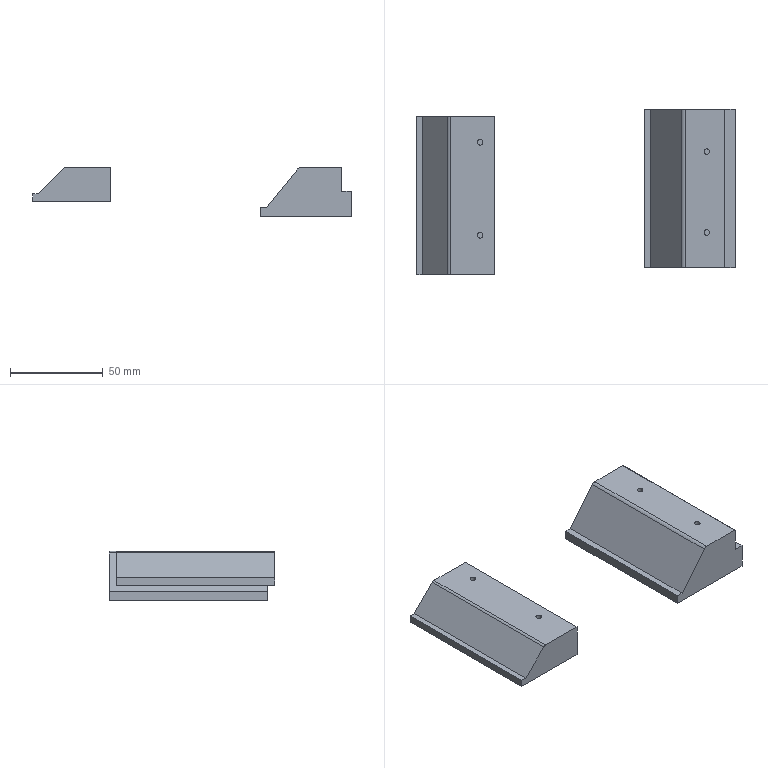Part | NX | 2 solids | 29 faces | box 171.319 x 88.841 x 26.598 mm | volume 135499 mm3 | plane 22 | cylinder 7 | commonest cylinder face diameters 3 x4 1 x1 4 x1 5 x1
STEP:
#1=CARTESIAN_POINT('',(92.218,-38.659,-21.598));
#2=VERTEX_POINT('',#1);
#3=CARTESIAN_POINT('',(92.218,-38.659,-26.598));
#4=VERTEX_POINT('',#3);
#5=CARTESIAN_POINT('',(92.218,-38.659,-21.598));
#6=DIRECTION('',(0.,0.,-1.));
#7=VECTOR('',#6,1000.);
#8=LINE('',#5,#7);
#9=EDGE_CURVE('',#2,#4,#8,.T.);
#10=ORIENTED_EDGE('',*,*,#9,.F.);
#11=CARTESIAN_POINT('',(92.218,46.341,-21.598));
#12=VERTEX_POINT('',#11);
#13=CARTESIAN_POINT('',(92.218,46.341,-21.598));
#14=DIRECTION('',(0.,-1.,0.));
#15=VECTOR('',#14,1000.);
#16=LINE('',#13,#15);
#17=EDGE_CURVE('',#12,#2,#16,.T.);
#18=ORIENTED_EDGE('',*,*,#17,.F.);
#19=CARTESIAN_POINT('',(92.218,46.341,-26.598));
#20=VERTEX_POINT('',#19);
#21=CARTESIAN_POINT('',(92.218,46.341,-21.598));
#22=DIRECTION('',(0.,0.,-1.));
#23=VECTOR('',#22,1000.);
#24=LINE('',#21,#23);
#25=EDGE_CURVE('',#12,#20,#24,.T.);
#26=ORIENTED_EDGE('',*,*,#25,.T.);
#27=CARTESIAN_POINT('',(92.218,46.341,-26.598));
#28=DIRECTION('',(0.,-1.,0.));
#29=VECTOR('',#28,1000.);
#30=LINE('',#27,#29);
#31=EDGE_CURVE('',#20,#4,#30,.T.);
#32=ORIENTED_EDGE('',*,*,#31,.T.);
#33=EDGE_LOOP('',(#10,#18,#26,#32));
#34=FACE_BOUND('',#33,.T.);
#35=CARTESIAN_POINT('',(92.218,46.341,-21.598));
#36=DIRECTION('',(-1.,0.,0.));
#37=DIRECTION('',(0.,-1.,0.));
#38=AXIS2_PLACEMENT_3D('',#35,#36,#37);
#39=PLANE('',#38);
#40=ADVANCED_FACE('',(#34),#39,.T.);
#41=CARTESIAN_POINT('',(141.218,-38.659,-26.598));
#42=VERTEX_POINT('',#41);
#43=CARTESIAN_POINT('',(92.218,-38.659,-26.598));
#44=DIRECTION('',(1.,0.,0.));
#45=VECTOR('',#44,1000.);
#46=LINE('',#43,#45);
#47=EDGE_CURVE('',#4,#42,#46,.T.);
#48=ORIENTED_EDGE('',*,*,#47,.F.);
#49=ORIENTED_EDGE('',*,*,#31,.F.);
#50=CARTESIAN_POINT('',(141.218,46.341,-26.598));
#51=VERTEX_POINT('',#50);
#52=CARTESIAN_POINT('',(92.218,46.341,-26.598));
#53=DIRECTION('',(1.,0.,0.));
#54=VECTOR('',#53,1000.);
#55=LINE('',#52,#54);
#56=EDGE_CURVE('',#20,#51,#55,.T.);
#57=ORIENTED_EDGE('',*,*,#56,.T.);
#58=CARTESIAN_POINT('',(141.218,46.341,-26.598));
#59=DIRECTION('',(0.,-1.,0.));
#60=VECTOR('',#59,1000.);
#61=LINE('',#58,#60);
#62=EDGE_CURVE('',#51,#42,#61,.T.);
#63=ORIENTED_EDGE('',*,*,#62,.T.);
#64=EDGE_LOOP('',(#48,#49,#57,#63));
#65=FACE_BOUND('',#64,.T.);
#66=CARTESIAN_POINT('',(92.218,46.341,-26.598));
#67=DIRECTION('',(0.,0.,-1.));
#68=DIRECTION('',(0.,1.,0.));
#69=AXIS2_PLACEMENT_3D('',#66,#67,#68);
#70=PLANE('',#69);
#71=ADVANCED_FACE('',(#65),#70,.T.);
#72=CARTESIAN_POINT('',(141.218,-38.659,-13.));
#73=VERTEX_POINT('',#72);
#74=CARTESIAN_POINT('',(141.218,-38.659,-26.598));
#75=DIRECTION('',(0.,0.,1.));
#76=VECTOR('',#75,1000.);
#77=LINE('',#74,#76);
#78=EDGE_CURVE('',#42,#73,#77,.T.);
#79=ORIENTED_EDGE('',*,*,#78,.F.);
#80=ORIENTED_EDGE('',*,*,#62,.F.);
#81=CARTESIAN_POINT('',(141.218,46.341,-13.));
#82=VERTEX_POINT('',#81);
#83=CARTESIAN_POINT('',(141.218,46.341,-26.598));
#84=DIRECTION('',(0.,0.,1.));
#85=VECTOR('',#84,1000.);
#86=LINE('',#83,#85);
#87=EDGE_CURVE('',#51,#82,#86,.T.);
#88=ORIENTED_EDGE('',*,*,#87,.T.);
#89=CARTESIAN_POINT('',(141.218,46.341,-13.));
#90=DIRECTION('',(0.,-1.,0.));
#91=VECTOR('',#90,1000.);
#92=LINE('',#89,#91);
#93=EDGE_CURVE('',#82,#73,#92,.T.);
#94=ORIENTED_EDGE('',*,*,#93,.T.);
#95=EDGE_LOOP('',(#79,#80,#88,#94));
#96=FACE_BOUND('',#95,.T.);
#97=CARTESIAN_POINT('',(141.218,46.341,-26.598));
#98=DIRECTION('',(1.,0.,0.));
#99=DIRECTION('',(0.,1.,0.));
#100=AXIS2_PLACEMENT_3D('',#97,#98,#99);
#101=PLANE('',#100);
#102=ADVANCED_FACE('',(#96),#101,.T.);
#103=CARTESIAN_POINT('',(136.064,-38.659,-13.));
#104=VERTEX_POINT('',#103);
#105=CARTESIAN_POINT('',(141.218,-38.659,-13.));
#106=DIRECTION('',(-1.,0.,0.));
#107=VECTOR('',#106,1000.);
#108=LINE('',#105,#107);
#109=EDGE_CURVE('',#73,#104,#108,.T.);
#110=ORIENTED_EDGE('',*,*,#109,.F.);
#111=ORIENTED_EDGE('',*,*,#93,.F.);
#112=CARTESIAN_POINT('',(136.064,46.341,-13.));
#113=VERTEX_POINT('',#112);
#114=CARTESIAN_POINT('',(141.218,46.341,-13.));
#115=DIRECTION('',(-1.,0.,0.));
#116=VECTOR('',#115,1000.);
#117=LINE('',#114,#116);
#118=EDGE_CURVE('',#82,#113,#117,.T.);
#119=ORIENTED_EDGE('',*,*,#118,.T.);
#120=CARTESIAN_POINT('',(136.064,46.341,-13.));
#121=DIRECTION('',(0.,-1.,0.));
#122=VECTOR('',#121,1000.);
#123=LINE('',#120,#122);
#124=EDGE_CURVE('',#113,#104,#123,.T.);
#125=ORIENTED_EDGE('',*,*,#124,.T.);
#126=EDGE_LOOP('',(#110,#111,#119,#125));
#127=FACE_BOUND('',#126,.T.);
#128=CARTESIAN_POINT('',(141.218,46.341,-13.));
#129=DIRECTION('',(0.,0.,1.));
#130=DIRECTION('',(0.,-1.,0.));
#131=AXIS2_PLACEMENT_3D('',#128,#129,#130);
#132=PLANE('',#131);
#133=ADVANCED_FACE('',(#127),#132,.T.);
#134=CARTESIAN_POINT('',(136.064,-38.659,-0.5));
#135=VERTEX_POINT('',#134);
#136=CARTESIAN_POINT('',(136.064,-38.659,-13.));
#137=DIRECTION('',(0.,0.,1.));
#138=VECTOR('',#137,1000.);
#139=LINE('',#136,#138);
#140=EDGE_CURVE('',#104,#135,#139,.T.);
#141=ORIENTED_EDGE('',*,*,#140,.F.);
#142=ORIENTED_EDGE('',*,*,#124,.F.);
#143=CARTESIAN_POINT('',(136.064,46.341,-0.5));
#144=VERTEX_POINT('',#143);
#145=CARTESIAN_POINT('',(136.064,46.341,-13.));
#146=DIRECTION('',(0.,0.,1.));
#147=VECTOR('',#146,1000.);
#148=LINE('',#145,#147);
#149=EDGE_CURVE('',#113,#144,#148,.T.);
#150=ORIENTED_EDGE('',*,*,#149,.T.);
#151=CARTESIAN_POINT('',(136.064,46.341,-0.5));
#152=DIRECTION('',(0.,-1.,0.));
#153=VECTOR('',#152,1000.);
#154=LINE('',#151,#153);
#155=EDGE_CURVE('',#144,#135,#154,.T.);
#156=ORIENTED_EDGE('',*,*,#155,.T.);
#157=EDGE_LOOP('',(#141,#142,#150,#156));
#158=FACE_BOUND('',#157,.T.);
#159=CARTESIAN_POINT('',(136.064,46.341,-13.));
#160=DIRECTION('',(1.,0.,0.));
#161=DIRECTION('',(0.,1.,0.));
#162=AXIS2_PLACEMENT_3D('',#159,#160,#161);
#163=PLANE('',#162);
#164=ADVANCED_FACE('',(#158),#163,.T.);
#165=CARTESIAN_POINT('',(135.564,-38.659,0.));
#166=VERTEX_POINT('',#165);
#167=CARTESIAN_POINT('',(135.564,-38.659,-0.5));
#168=DIRECTION('',(0.,-1.,0.));
#169=DIRECTION('',(1.,0.,0.));
#170=AXIS2_PLACEMENT_3D('',#167,#168,#169);
#171=CIRCLE('',#170,0.5);
#172=EDGE_CURVE('',#135,#166,#171,.T.);
#173=ORIENTED_EDGE('',*,*,#172,.F.);
#174=ORIENTED_EDGE('',*,*,#155,.F.);
#175=CARTESIAN_POINT('',(135.564,46.341,0.));
#176=VERTEX_POINT('',#175);
#177=CARTESIAN_POINT('',(135.564,46.341,-0.5));
#178=DIRECTION('',(0.,-1.,0.));
#179=DIRECTION('',(1.,0.,0.));
#180=AXIS2_PLACEMENT_3D('',#177,#178,#179);
#181=CIRCLE('',#180,0.5);
#182=EDGE_CURVE('',#144,#176,#181,.T.);
#183=ORIENTED_EDGE('',*,*,#182,.T.);
#184=CARTESIAN_POINT('',(135.564,46.341,0.));
#185=DIRECTION('',(0.,-1.,0.));
#186=VECTOR('',#185,1000.);
#187=LINE('',#184,#186);
#188=EDGE_CURVE('',#176,#166,#187,.T.);
#189=ORIENTED_EDGE('',*,*,#188,.T.);
#190=EDGE_LOOP('',(#173,#174,#183,#189));
#191=FACE_BOUND('',#190,.T.);
#192=CARTESIAN_POINT('',(135.564,46.341,-0.5));
#193=DIRECTION('',(0.,-1.,0.));
#194=DIRECTION('',(1.,0.,0.));
#195=AXIS2_PLACEMENT_3D('',#192,#193,#194);
#196=CYLINDRICAL_SURFACE('',#195,0.5);
#197=ADVANCED_FACE('',(#191),#196,.T.);
#198=CARTESIAN_POINT('',(127.424,23.591,0.));
#199=VERTEX_POINT('',#198);
#200=CARTESIAN_POINT('',(125.924,23.591,0.));
#201=DIRECTION('',(0.,0.,1.));
#202=DIRECTION('',(1.,0.,0.));
#203=AXIS2_PLACEMENT_3D('',#200,#201,#202);
#204=CIRCLE('',#203,1.5);
#205=EDGE_CURVE('',#199,#199,#204,.T.);
#206=ORIENTED_EDGE('',*,*,#205,.F.);
#207=EDGE_LOOP('',(#206));
#208=FACE_BOUND('',#207,.T.);
#209=CARTESIAN_POINT('',(127.424,-19.908,0.));
#210=VERTEX_POINT('',#209);
#211=CARTESIAN_POINT('',(125.924,-19.908,0.));
#212=DIRECTION('',(0.,0.,1.));
#213=DIRECTION('',(1.,0.,0.));
#214=AXIS2_PLACEMENT_3D('',#211,#212,#213);
#215=CIRCLE('',#214,1.5);
#216=EDGE_CURVE('',#210,#210,#215,.T.);
#217=ORIENTED_EDGE('',*,*,#216,.F.);
#218=EDGE_LOOP('',(#217));
#219=FACE_BOUND('',#218,.T.);
#220=CARTESIAN_POINT('',(114.318,-38.659,0.));
#221=VERTEX_POINT('',#220);
#222=CARTESIAN_POINT('',(135.564,-38.659,0.));
#223=DIRECTION('',(-1.,0.,0.));
#224=VECTOR('',#223,1000.);
#225=LINE('',#222,#224);
#226=EDGE_CURVE('',#166,#221,#225,.T.);
#227=ORIENTED_EDGE('',*,*,#226,.F.);
#228=ORIENTED_EDGE('',*,*,#188,.F.);
#229=CARTESIAN_POINT('',(114.318,46.341,0.));
#230=VERTEX_POINT('',#229);
#231=CARTESIAN_POINT('',(135.564,46.341,0.));
#232=DIRECTION('',(-1.,0.,0.));
#233=VECTOR('',#232,1000.);
#234=LINE('',#231,#233);
#235=EDGE_CURVE('',#176,#230,#234,.T.);
#236=ORIENTED_EDGE('',*,*,#235,.T.);
#237=CARTESIAN_POINT('',(114.318,46.341,0.));
#238=DIRECTION('',(0.,-1.,0.));
#239=VECTOR('',#238,1000.);
#240=LINE('',#237,#239);
#241=EDGE_CURVE('',#230,#221,#240,.T.);
#242=ORIENTED_EDGE('',*,*,#241,.T.);
#243=EDGE_LOOP('',(#227,#228,#236,#242));
#244=FACE_BOUND('',#243,.T.);
#245=CARTESIAN_POINT('',(135.564,46.341,0.));
#246=DIRECTION('',(0.,0.,1.));
#247=DIRECTION('',(0.,-1.,0.));
#248=AXIS2_PLACEMENT_3D('',#245,#246,#247);
#249=PLANE('',#248);
#250=ADVANCED_FACE('',(#208,#219,#244),#249,.T.);
#251=CARTESIAN_POINT('',(112.375,-38.659,-0.9267));
#252=VERTEX_POINT('',#251);
#253=CARTESIAN_POINT('',(114.318,-38.659,-2.5));
#254=DIRECTION('',(0.,-1.,0.));
#255=DIRECTION('',(1.,0.,0.));
#256=AXIS2_PLACEMENT_3D('',#253,#254,#255);
#257=CIRCLE('',#256,2.5);
#258=EDGE_CURVE('',#221,#252,#257,.T.);
#259=ORIENTED_EDGE('',*,*,#258,.F.);
#260=ORIENTED_EDGE('',*,*,#241,.F.);
#261=CARTESIAN_POINT('',(112.375,46.341,-0.9267));
#262=VERTEX_POINT('',#261);
#263=CARTESIAN_POINT('',(114.318,46.341,-2.5));
#264=DIRECTION('',(0.,-1.,0.));
#265=DIRECTION('',(1.,0.,0.));
#266=AXIS2_PLACEMENT_3D('',#263,#264,#265);
#267=CIRCLE('',#266,2.5);
#268=EDGE_CURVE('',#230,#262,#267,.T.);
#269=ORIENTED_EDGE('',*,*,#268,.T.);
#270=CARTESIAN_POINT('',(112.375,46.341,-0.9267));
#271=DIRECTION('',(0.,-1.,0.));
#272=VECTOR('',#271,1000.);
#273=LINE('',#270,#272);
#274=EDGE_CURVE('',#262,#252,#273,.T.);
#275=ORIENTED_EDGE('',*,*,#274,.T.);
#276=EDGE_LOOP('',(#259,#260,#269,#275));
#277=FACE_BOUND('',#276,.T.);
#278=CARTESIAN_POINT('',(114.318,46.341,-2.5));
#279=DIRECTION('',(0.,-1.,0.));
#280=DIRECTION('',(1.,0.,0.));
#281=AXIS2_PLACEMENT_3D('',#278,#279,#280);
#282=CYLINDRICAL_SURFACE('',#281,2.5);
#283=ADVANCED_FACE('',(#277),#282,.T.);
#284=CARTESIAN_POINT('',(95.636,-38.659,-21.598));
#285=VERTEX_POINT('',#284);
#286=CARTESIAN_POINT('',(112.375,-38.659,-0.9267));
#287=DIRECTION('',(-0.6293,0.,-0.7771));
#288=VECTOR('',#287,1000.);
#289=LINE('',#286,#288);
#290=EDGE_CURVE('',#252,#285,#289,.T.);
#291=ORIENTED_EDGE('',*,*,#290,.F.);
#292=ORIENTED_EDGE('',*,*,#274,.F.);
#293=CARTESIAN_POINT('',(95.636,46.341,-21.598));
#294=VERTEX_POINT('',#293);
#295=CARTESIAN_POINT('',(112.375,46.341,-0.9267));
#296=DIRECTION('',(-0.6293,0.,-0.7771));
#297=VECTOR('',#296,1000.);
#298=LINE('',#295,#297);
#299=EDGE_CURVE('',#262,#294,#298,.T.);
#300=ORIENTED_EDGE('',*,*,#299,.T.);
#301=CARTESIAN_POINT('',(95.636,46.341,-21.598));
#302=DIRECTION('',(0.,-1.,0.));
#303=VECTOR('',#302,1000.);
#304=LINE('',#301,#303);
#305=EDGE_CURVE('',#294,#285,#304,.T.);
#306=ORIENTED_EDGE('',*,*,#305,.T.);
#307=EDGE_LOOP('',(#291,#292,#300,#306));
#308=FACE_BOUND('',#307,.T.);
#309=CARTESIAN_POINT('',(112.375,46.341,-0.9267));
#310=DIRECTION('',(-0.7771,0.,0.6293));
#311=DIRECTION('',(-0.6293,0.,-0.7771));
#312=AXIS2_PLACEMENT_3D('',#309,#310,#311);
#313=PLANE('',#312);
#314=ADVANCED_FACE('',(#308),#313,.T.);
#315=CARTESIAN_POINT('',(95.636,-38.659,-21.598));
#316=DIRECTION('',(-1.,0.,0.));
#317=VECTOR('',#316,1000.);
#318=LINE('',#315,#317);
#319=EDGE_CURVE('',#285,#2,#318,.T.);
#320=ORIENTED_EDGE('',*,*,#319,.F.);
#321=ORIENTED_EDGE('',*,*,#305,.F.);
#322=CARTESIAN_POINT('',(95.636,46.341,-21.598));
#323=DIRECTION('',(-1.,0.,0.));
#324=VECTOR('',#323,1000.);
#325=LINE('',#322,#324);
#326=EDGE_CURVE('',#294,#12,#325,.T.);
#327=ORIENTED_EDGE('',*,*,#326,.T.);
#328=ORIENTED_EDGE('',*,*,#17,.T.);
#329=EDGE_LOOP('',(#320,#321,#327,#328));
#330=FACE_BOUND('',#329,.T.);
#331=CARTESIAN_POINT('',(95.636,46.341,-21.598));
#332=DIRECTION('',(0.,0.,1.));
#333=DIRECTION('',(0.,-1.,0.));
#334=AXIS2_PLACEMENT_3D('',#331,#332,#333);
#335=PLANE('',#334);
#336=ADVANCED_FACE('',(#330),#335,.T.);
#337=ORIENTED_EDGE('',*,*,#25,.F.);
#338=ORIENTED_EDGE('',*,*,#326,.F.);
#339=ORIENTED_EDGE('',*,*,#299,.F.);
#340=ORIENTED_EDGE('',*,*,#268,.F.);
#341=ORIENTED_EDGE('',*,*,#235,.F.);
#342=ORIENTED_EDGE('',*,*,#182,.F.);
#343=ORIENTED_EDGE('',*,*,#149,.F.);
#344=ORIENTED_EDGE('',*,*,#118,.F.);
#345=ORIENTED_EDGE('',*,*,#87,.F.);
#346=ORIENTED_EDGE('',*,*,#56,.F.);
#347=EDGE_LOOP('',(#337,#338,#339,#340,#341,#342,#343,#344,#345,#346));
#348=FACE_BOUND('',#347,.T.);
#349=CARTESIAN_POINT('',(135.564,46.341,-0.5));
#350=DIRECTION('',(0.,-1.,0.));
#351=DIRECTION('',(1.,0.,0.));
#352=AXIS2_PLACEMENT_3D('',#349,#350,#351);
#353=PLANE('',#352);
#354=ADVANCED_FACE('',(#348),#353,.F.);
#355=ORIENTED_EDGE('',*,*,#9,.T.);
#356=ORIENTED_EDGE('',*,*,#47,.T.);
#357=ORIENTED_EDGE('',*,*,#78,.T.);
#358=ORIENTED_EDGE('',*,*,#109,.T.);
#359=ORIENTED_EDGE('',*,*,#140,.T.);
#360=ORIENTED_EDGE('',*,*,#172,.T.);
#361=ORIENTED_EDGE('',*,*,#226,.T.);
#362=ORIENTED_EDGE('',*,*,#258,.T.);
#363=ORIENTED_EDGE('',*,*,#290,.T.);
#364=ORIENTED_EDGE('',*,*,#319,.T.);
#365=EDGE_LOOP('',(#355,#356,#357,#358,#359,#360,#361,#362,#363,#364));
#366=FACE_BOUND('',#365,.T.);
#367=CARTESIAN_POINT('',(135.564,-38.659,-0.5));
#368=DIRECTION('',(0.,-1.,0.));
#369=DIRECTION('',(1.,0.,0.));
#370=AXIS2_PLACEMENT_3D('',#367,#368,#369);
#371=PLANE('',#370);
#372=ADVANCED_FACE('',(#366),#371,.T.);
#373=CARTESIAN_POINT('',(127.424,-19.908,-5.));
#374=VERTEX_POINT('',#373);
#375=CARTESIAN_POINT('',(125.924,-19.908,-5.));
#376=DIRECTION('',(0.,0.,1.));
#377=DIRECTION('',(1.,0.,0.));
#378=AXIS2_PLACEMENT_3D('',#375,#376,#377);
#379=CIRCLE('',#378,1.5);
#380=EDGE_CURVE('',#374,#374,#379,.F.);
#381=ORIENTED_EDGE('',*,*,#380,.T.);
#382=EDGE_LOOP('',(#381));
#383=FACE_BOUND('',#382,.T.);
#384=ORIENTED_EDGE('',*,*,#216,.T.);
#385=EDGE_LOOP('',(#384));
#386=FACE_BOUND('',#385,.T.);
#387=CARTESIAN_POINT('',(125.924,-19.908,-5.));
#388=DIRECTION('',(0.,0.,1.));
#389=DIRECTION('',(1.,0.,0.));
#390=AXIS2_PLACEMENT_3D('',#387,#388,#389);
#391=CYLINDRICAL_SURFACE('',#390,1.5);
#392=ADVANCED_FACE('',(#383,#386),#391,.F.);
#393=ORIENTED_EDGE('',*,*,#380,.F.);
#394=EDGE_LOOP('',(#393));
#395=FACE_BOUND('',#394,.T.);
#396=CARTESIAN_POINT('',(125.924,-19.908,-5.));
#397=DIRECTION('',(0.,0.,1.));
#398=DIRECTION('',(1.,0.,0.));
#399=AXIS2_PLACEMENT_3D('',#396,#397,#398);
#400=PLANE('',#399);
#401=ADVANCED_FACE('',(#395),#400,.T.);
#402=CARTESIAN_POINT('',(127.424,23.591,-5.));
#403=VERTEX_POINT('',#402);
#404=CARTESIAN_POINT('',(125.924,23.591,-5.));
#405=DIRECTION('',(0.,0.,1.));
#406=DIRECTION('',(1.,0.,0.));
#407=AXIS2_PLACEMENT_3D('',#404,#405,#406);
#408=CIRCLE('',#407,1.5);
#409=EDGE_CURVE('',#403,#403,#408,.F.);
#410=ORIENTED_EDGE('',*,*,#409,.T.);
#411=EDGE_LOOP('',(#410));
#412=FACE_BOUND('',#411,.T.);
#413=ORIENTED_EDGE('',*,*,#205,.T.);
#414=EDGE_LOOP('',(#413));
#415=FACE_BOUND('',#414,.T.);
#416=CARTESIAN_POINT('',(125.924,23.591,-5.));
#417=DIRECTION('',(0.,0.,1.));
#418=DIRECTION('',(1.,0.,0.));
#419=AXIS2_PLACEMENT_3D('',#416,#417,#418);
#420=CYLINDRICAL_SURFACE('',#419,1.5);
#421=ADVANCED_FACE('',(#412,#415),#420,.F.);
#422=ORIENTED_EDGE('',*,*,#409,.F.);
#423=EDGE_LOOP('',(#422));
#424=FACE_BOUND('',#423,.T.);
#425=CARTESIAN_POINT('',(125.924,23.591,-5.));
#426=DIRECTION('',(0.,0.,1.));
#427=DIRECTION('',(1.,0.,0.));
#428=AXIS2_PLACEMENT_3D('',#425,#426,#427);
#429=PLANE('',#428);
#430=ADVANCED_FACE('',(#424),#429,.T.);
#431=CLOSED_SHELL('',(#40,#71,#102,#133,#164,#197,#250,#283,#314,#336,#354,#372,#392,#401,#421,#430));
#432=MANIFOLD_SOLID_BREP('',#431);
#433=CARTESIAN_POINT('',(-13.313,-42.5,-0.5858));
#434=VERTEX_POINT('',#433);
#435=CARTESIAN_POINT('',(-27.03,-42.5,-14.302));
#436=VERTEX_POINT('',#435);
#437=CARTESIAN_POINT('',(-13.313,-42.5,-0.5858));
#438=DIRECTION('',(-0.7071,0.,-0.7071));
#439=VECTOR('',#438,1000.);
#440=LINE('',#437,#439);
#441=EDGE_CURVE('',#434,#436,#440,.T.);
#442=ORIENTED_EDGE('',*,*,#441,.F.);
#443=CARTESIAN_POINT('',(-13.313,42.5,-0.5858));
#444=VERTEX_POINT('',#443);
#445=CARTESIAN_POINT('',(-13.313,42.5,-0.5858));
#446=DIRECTION('',(0.,-1.,0.));
#447=VECTOR('',#446,1000.);
#448=LINE('',#445,#447);
#449=EDGE_CURVE('',#444,#434,#448,.T.);
#450=ORIENTED_EDGE('',*,*,#449,.F.);
#451=CARTESIAN_POINT('',(-27.03,42.5,-14.302));
#452=VERTEX_POINT('',#451);
#453=CARTESIAN_POINT('',(-13.313,42.5,-0.5858));
#454=DIRECTION('',(-0.7071,0.,-0.7071));
#455=VECTOR('',#454,1000.);
#456=LINE('',#453,#455);
#457=EDGE_CURVE('',#444,#452,#456,.T.);
#458=ORIENTED_EDGE('',*,*,#457,.T.);
#459=CARTESIAN_POINT('',(-27.03,42.5,-14.302));
#460=DIRECTION('',(0.,-1.,0.));
#461=VECTOR('',#460,1000.);
#462=LINE('',#459,#461);
#463=EDGE_CURVE('',#452,#436,#462,.T.);
#464=ORIENTED_EDGE('',*,*,#463,.T.);
#465=EDGE_LOOP('',(#442,#450,#458,#464));
#466=FACE_BOUND('',#465,.T.);
#467=CARTESIAN_POINT('',(-13.313,42.5,-0.5858));
#468=DIRECTION('',(-0.7071,0.,0.7071));
#469=DIRECTION('',(-0.7071,0.,-0.7071));
#470=AXIS2_PLACEMENT_3D('',#467,#468,#469);
#471=PLANE('',#470);
#472=ADVANCED_FACE('',(#466),#471,.T.);
#473=CARTESIAN_POINT('',(-30.101,-42.5,-14.302));
#474=VERTEX_POINT('',#473);
#475=CARTESIAN_POINT('',(-27.03,-42.5,-14.302));
#476=DIRECTION('',(-1.,0.,0.));
#477=VECTOR('',#476,1000.);
#478=LINE('',#475,#477);
#479=EDGE_CURVE('',#436,#474,#478,.T.);
#480=ORIENTED_EDGE('',*,*,#479,.F.);
#481=ORIENTED_EDGE('',*,*,#463,.F.);
#482=CARTESIAN_POINT('',(-30.101,42.5,-14.302));
#483=VERTEX_POINT('',#482);
#484=CARTESIAN_POINT('',(-27.03,42.5,-14.302));
#485=DIRECTION('',(-1.,0.,0.));
#486=VECTOR('',#485,1000.);
#487=LINE('',#484,#486);
#488=EDGE_CURVE('',#452,#483,#487,.T.);
#489=ORIENTED_EDGE('',*,*,#488,.T.);
#490=CARTESIAN_POINT('',(-30.101,42.5,-14.302));
#491=DIRECTION('',(0.,-1.,0.));
#492=VECTOR('',#491,1000.);
#493=LINE('',#490,#492);
#494=EDGE_CURVE('',#483,#474,#493,.T.);
#495=ORIENTED_EDGE('',*,*,#494,.T.);
#496=EDGE_LOOP('',(#480,#481,#489,#495));
#497=FACE_BOUND('',#496,.T.);
#498=CARTESIAN_POINT('',(-27.03,42.5,-14.302));
#499=DIRECTION('',(0.,0.,1.));
#500=DIRECTION('',(0.,-1.,0.));
#501=AXIS2_PLACEMENT_3D('',#498,#499,#500);
#502=PLANE('',#501);
#503=ADVANCED_FACE('',(#497),#502,.T.);
#504=CARTESIAN_POINT('',(-30.101,-42.5,-18.302));
#505=VERTEX_POINT('',#504);
#506=CARTESIAN_POINT('',(-30.101,-42.5,-14.302));
#507=DIRECTION('',(0.,0.,-1.));
#508=VECTOR('',#507,1000.);
#509=LINE('',#506,#508);
#510=EDGE_CURVE('',#474,#505,#509,.T.);
#511=ORIENTED_EDGE('',*,*,#510,.F.);
#512=ORIENTED_EDGE('',*,*,#494,.F.);
#513=CARTESIAN_POINT('',(-30.101,42.5,-18.302));
#514=VERTEX_POINT('',#513);
#515=CARTESIAN_POINT('',(-30.101,42.5,-14.302));
#516=DIRECTION('',(0.,0.,-1.));
#517=VECTOR('',#516,1000.);
#518=LINE('',#515,#517);
#519=EDGE_CURVE('',#483,#514,#518,.T.);
#520=ORIENTED_EDGE('',*,*,#519,.T.);
#521=CARTESIAN_POINT('',(-30.101,42.5,-18.302));
#522=DIRECTION('',(0.,-1.,0.));
#523=VECTOR('',#522,1000.);
#524=LINE('',#521,#523);
#525=EDGE_CURVE('',#514,#505,#524,.T.);
#526=ORIENTED_EDGE('',*,*,#525,.T.);
#527=EDGE_LOOP('',(#511,#512,#520,#526));
#528=FACE_BOUND('',#527,.T.);
#529=CARTESIAN_POINT('',(-30.101,42.5,-14.302));
#530=DIRECTION('',(-1.,0.,0.));
#531=DIRECTION('',(0.,-1.,0.));
#532=AXIS2_PLACEMENT_3D('',#529,#530,#531);
#533=PLANE('',#532);
#534=ADVANCED_FACE('',(#528),#533,.T.);
#535=CARTESIAN_POINT('',(11.899,-42.5,-18.302));
#536=VERTEX_POINT('',#535);
#537=CARTESIAN_POINT('',(-30.101,-42.5,-18.302));
#538=DIRECTION('',(1.,0.,0.));
#539=VECTOR('',#538,1000.);
#540=LINE('',#537,#539);
#541=EDGE_CURVE('',#505,#536,#540,.T.);
#542=ORIENTED_EDGE('',*,*,#541,.F.);
#543=ORIENTED_EDGE('',*,*,#525,.F.);
#544=CARTESIAN_POINT('',(11.899,42.5,-18.302));
#545=VERTEX_POINT('',#544);
#546=CARTESIAN_POINT('',(-30.101,42.5,-18.302));
#547=DIRECTION('',(1.,0.,0.));
#548=VECTOR('',#547,1000.);
#549=LINE('',#546,#548);
#550=EDGE_CURVE('',#514,#545,#549,.T.);
#551=ORIENTED_EDGE('',*,*,#550,.T.);
#552=CARTESIAN_POINT('',(11.899,42.5,-18.302));
#553=DIRECTION('',(0.,-1.,0.));
#554=VECTOR('',#553,1000.);
#555=LINE('',#552,#554);
#556=EDGE_CURVE('',#545,#536,#555,.T.);
#557=ORIENTED_EDGE('',*,*,#556,.T.);
#558=EDGE_LOOP('',(#542,#543,#551,#557));
#559=FACE_BOUND('',#558,.T.);
#560=CARTESIAN_POINT('',(-30.101,42.5,-18.302));
#561=DIRECTION('',(0.,0.,-1.));
#562=DIRECTION('',(0.,1.,0.));
#563=AXIS2_PLACEMENT_3D('',#560,#561,#562);
#564=PLANE('',#563);
#565=ADVANCED_FACE('',(#559),#564,.T.);
#566=CARTESIAN_POINT('',(11.899,-42.5,0.));
#567=VERTEX_POINT('',#566);
#568=CARTESIAN_POINT('',(11.899,-42.5,-18.302));
#569=DIRECTION('',(0.,0.,1.));
#570=VECTOR('',#569,1000.);
#571=LINE('',#568,#570);
#572=EDGE_CURVE('',#536,#567,#571,.T.);
#573=ORIENTED_EDGE('',*,*,#572,.F.);
#574=ORIENTED_EDGE('',*,*,#556,.F.);
#575=CARTESIAN_POINT('',(11.899,42.5,0.));
#576=VERTEX_POINT('',#575);
#577=CARTESIAN_POINT('',(11.899,42.5,-18.302));
#578=DIRECTION('',(0.,0.,1.));
#579=VECTOR('',#578,1000.);
#580=LINE('',#577,#579);
#581=EDGE_CURVE('',#545,#576,#580,.T.);
#582=ORIENTED_EDGE('',*,*,#581,.T.);
#583=CARTESIAN_POINT('',(11.899,42.5,0.));
#584=DIRECTION('',(0.,-1.,0.));
#585=VECTOR('',#584,1000.);
#586=LINE('',#583,#585);
#587=EDGE_CURVE('',#576,#567,#586,.T.);
#588=ORIENTED_EDGE('',*,*,#587,.T.);
#589=EDGE_LOOP('',(#573,#574,#582,#588));
#590=FACE_BOUND('',#589,.T.);
#591=CARTESIAN_POINT('',(11.899,42.5,-18.302));
#592=DIRECTION('',(1.,0.,0.));
#593=DIRECTION('',(0.,1.,0.));
#594=AXIS2_PLACEMENT_3D('',#591,#592,#593);
#595=PLANE('',#594);
#596=ADVANCED_FACE('',(#590),#595,.T.);
#597=CARTESIAN_POINT('',(5.485,28.65,0.));
#598=VERTEX_POINT('',#597);
#599=CARTESIAN_POINT('',(3.985,28.65,0.));
#600=DIRECTION('',(0.,0.,1.));
#601=DIRECTION('',(1.,0.,0.));
#602=AXIS2_PLACEMENT_3D('',#599,#600,#601);
#603=CIRCLE('',#602,1.5);
#604=EDGE_CURVE('',#598,#598,#603,.T.);
#605=ORIENTED_EDGE('',*,*,#604,.F.);
#606=EDGE_LOOP('',(#605));
#607=FACE_BOUND('',#606,.T.);
#608=CARTESIAN_POINT('',(5.485,-21.35,0.));
#609=VERTEX_POINT('',#608);
#610=CARTESIAN_POINT('',(3.985,-21.35,0.));
#611=DIRECTION('',(0.,0.,1.));
#612=DIRECTION('',(1.,0.,0.));
#613=AXIS2_PLACEMENT_3D('',#610,#611,#612);
#614=CIRCLE('',#613,1.5);
#615=EDGE_CURVE('',#609,#609,#614,.T.);
#616=ORIENTED_EDGE('',*,*,#615,.F.);
#617=EDGE_LOOP('',(#616));
#618=FACE_BOUND('',#617,.T.);
#619=CARTESIAN_POINT('',(-11.899,-42.5,0.));
#620=VERTEX_POINT('',#619);
#621=CARTESIAN_POINT('',(11.899,-42.5,0.));
#622=DIRECTION('',(-1.,0.,0.));
#623=VECTOR('',#622,1000.);
#624=LINE('',#621,#623);
#625=EDGE_CURVE('',#567,#620,#624,.T.);
#626=ORIENTED_EDGE('',*,*,#625,.F.);
#627=ORIENTED_EDGE('',*,*,#587,.F.);
#628=CARTESIAN_POINT('',(-11.899,42.5,0.));
#629=VERTEX_POINT('',#628);
#630=CARTESIAN_POINT('',(11.899,42.5,0.));
#631=DIRECTION('',(-1.,0.,0.));
#632=VECTOR('',#631,1000.);
#633=LINE('',#630,#632);
#634=EDGE_CURVE('',#576,#629,#633,.T.);
#635=ORIENTED_EDGE('',*,*,#634,.T.);
#636=CARTESIAN_POINT('',(-11.899,42.5,0.));
#637=DIRECTION('',(0.,-1.,0.));
#638=VECTOR('',#637,1000.);
#639=LINE('',#636,#638);
#640=EDGE_CURVE('',#629,#620,#639,.T.);
#641=ORIENTED_EDGE('',*,*,#640,.T.);
#642=EDGE_LOOP('',(#626,#627,#635,#641));
#643=FACE_BOUND('',#642,.T.);
#644=CARTESIAN_POINT('',(11.899,42.5,0.));
#645=DIRECTION('',(0.,0.,1.));
#646=DIRECTION('',(0.,-1.,0.));
#647=AXIS2_PLACEMENT_3D('',#644,#645,#646);
#648=PLANE('',#647);
#649=ADVANCED_FACE('',(#607,#618,#643),#648,.T.);
#650=CARTESIAN_POINT('',(-11.899,-42.5,-2.));
#651=DIRECTION('',(0.,-1.,0.));
#652=DIRECTION('',(1.,0.,0.));
#653=AXIS2_PLACEMENT_3D('',#650,#651,#652);
#654=CIRCLE('',#653,2.);
#655=EDGE_CURVE('',#620,#434,#654,.T.);
#656=ORIENTED_EDGE('',*,*,#655,.F.);
#657=ORIENTED_EDGE('',*,*,#640,.F.);
#658=CARTESIAN_POINT('',(-11.899,42.5,-2.));
#659=DIRECTION('',(0.,-1.,0.));
#660=DIRECTION('',(1.,0.,0.));
#661=AXIS2_PLACEMENT_3D('',#658,#659,#660);
#662=CIRCLE('',#661,2.);
#663=EDGE_CURVE('',#629,#444,#662,.T.);
#664=ORIENTED_EDGE('',*,*,#663,.T.);
#665=ORIENTED_EDGE('',*,*,#449,.T.);
#666=EDGE_LOOP('',(#656,#657,#664,#665));
#667=FACE_BOUND('',#666,.T.);
#668=CARTESIAN_POINT('',(-11.899,42.5,-2.));
#669=DIRECTION('',(0.,-1.,0.));
#670=DIRECTION('',(1.,0.,0.));
#671=AXIS2_PLACEMENT_3D('',#668,#669,#670);
#672=CYLINDRICAL_SURFACE('',#671,2.);
#673=ADVANCED_FACE('',(#667),#672,.T.);
#674=ORIENTED_EDGE('',*,*,#457,.F.);
#675=ORIENTED_EDGE('',*,*,#663,.F.);
#676=ORIENTED_EDGE('',*,*,#634,.F.);
#677=ORIENTED_EDGE('',*,*,#581,.F.);
#678=ORIENTED_EDGE('',*,*,#550,.F.);
#679=ORIENTED_EDGE('',*,*,#519,.F.);
#680=ORIENTED_EDGE('',*,*,#488,.F.);
#681=EDGE_LOOP('',(#674,#675,#676,#677,#678,#679,#680));
#682=FACE_BOUND('',#681,.T.);
#683=CARTESIAN_POINT('',(-11.899,42.5,-2.));
#684=DIRECTION('',(0.,-1.,0.));
#685=DIRECTION('',(1.,0.,0.));
#686=AXIS2_PLACEMENT_3D('',#683,#684,#685);
#687=PLANE('',#686);
#688=ADVANCED_FACE('',(#682),#687,.F.);
#689=ORIENTED_EDGE('',*,*,#441,.T.);
#690=ORIENTED_EDGE('',*,*,#479,.T.);
#691=ORIENTED_EDGE('',*,*,#510,.T.);
#692=ORIENTED_EDGE('',*,*,#541,.T.);
#693=ORIENTED_EDGE('',*,*,#572,.T.);
#694=ORIENTED_EDGE('',*,*,#625,.T.);
#695=ORIENTED_EDGE('',*,*,#655,.T.);
#696=EDGE_LOOP('',(#689,#690,#691,#692,#693,#694,#695));
#697=FACE_BOUND('',#696,.T.);
#698=CARTESIAN_POINT('',(-11.899,-42.5,-2.));
#699=DIRECTION('',(0.,-1.,0.));
#700=DIRECTION('',(1.,0.,0.));
#701=AXIS2_PLACEMENT_3D('',#698,#699,#700);
#702=PLANE('',#701);
#703=ADVANCED_FACE('',(#697),#702,.T.);
#704=CARTESIAN_POINT('',(5.485,-21.35,-5.));
#705=VERTEX_POINT('',#704);
#706=CARTESIAN_POINT('',(3.985,-21.35,-5.));
#707=DIRECTION('',(0.,0.,1.));
#708=DIRECTION('',(1.,0.,0.));
#709=AXIS2_PLACEMENT_3D('',#706,#707,#708);
#710=CIRCLE('',#709,1.5);
#711=EDGE_CURVE('',#705,#705,#710,.F.);
#712=ORIENTED_EDGE('',*,*,#711,.T.);
#713=EDGE_LOOP('',(#712));
#714=FACE_BOUND('',#713,.T.);
#715=ORIENTED_EDGE('',*,*,#615,.T.);
#716=EDGE_LOOP('',(#715));
#717=FACE_BOUND('',#716,.T.);
#718=CARTESIAN_POINT('',(3.985,-21.35,-5.));
#719=DIRECTION('',(0.,0.,1.));
#720=DIRECTION('',(1.,0.,0.));
#721=AXIS2_PLACEMENT_3D('',#718,#719,#720);
#722=CYLINDRICAL_SURFACE('',#721,1.5);
#723=ADVANCED_FACE('',(#714,#717),#722,.F.);
#724=ORIENTED_EDGE('',*,*,#711,.F.);
#725=EDGE_LOOP('',(#724));
#726=FACE_BOUND('',#725,.T.);
#727=CARTESIAN_POINT('',(3.985,-21.35,-5.));
#728=DIRECTION('',(0.,0.,1.));
#729=DIRECTION('',(1.,0.,0.));
#730=AXIS2_PLACEMENT_3D('',#727,#728,#729);
#731=PLANE('',#730);
#732=ADVANCED_FACE('',(#726),#731,.T.);
#733=CARTESIAN_POINT('',(5.485,28.65,-5.));
#734=VERTEX_POINT('',#733);
#735=CARTESIAN_POINT('',(3.985,28.65,-5.));
#736=DIRECTION('',(0.,0.,1.));
#737=DIRECTION('',(1.,0.,0.));
#738=AXIS2_PLACEMENT_3D('',#735,#736,#737);
#739=CIRCLE('',#738,1.5);
#740=EDGE_CURVE('',#734,#734,#739,.F.);
#741=ORIENTED_EDGE('',*,*,#740,.T.);
#742=EDGE_LOOP('',(#741));
#743=FACE_BOUND('',#742,.T.);
#744=ORIENTED_EDGE('',*,*,#604,.T.);
#745=EDGE_LOOP('',(#744));
#746=FACE_BOUND('',#745,.T.);
#747=CARTESIAN_POINT('',(3.985,28.65,-5.));
#748=DIRECTION('',(0.,0.,1.));
#749=DIRECTION('',(1.,0.,0.));
#750=AXIS2_PLACEMENT_3D('',#747,#748,#749);
#751=CYLINDRICAL_SURFACE('',#750,1.5);
#752=ADVANCED_FACE('',(#743,#746),#751,.F.);
#753=ORIENTED_EDGE('',*,*,#740,.F.);
#754=EDGE_LOOP('',(#753));
#755=FACE_BOUND('',#754,.T.);
#756=CARTESIAN_POINT('',(3.985,28.65,-5.));
#757=DIRECTION('',(0.,0.,1.));
#758=DIRECTION('',(1.,0.,0.));
#759=AXIS2_PLACEMENT_3D('',#756,#757,#758);
#760=PLANE('',#759);
#761=ADVANCED_FACE('',(#755),#760,.T.);
#762=CLOSED_SHELL('',(#472,#503,#534,#565,#596,#649,#673,#688,#703,#723,#732,#752,#761));
#763=MANIFOLD_SOLID_BREP('',#762);
#764=(LENGTH_UNIT()NAMED_UNIT(*)SI_UNIT(.MILLI.,.METRE.));
#765=UNCERTAINTY_MEASURE_WITH_UNIT(LENGTH_MEASURE(0.00001),#764,'','');
#766=(NAMED_UNIT(*)PLANE_ANGLE_UNIT()SI_UNIT($,.RADIAN.));
#767=(NAMED_UNIT(*)SI_UNIT($,.STERADIAN.)SOLID_ANGLE_UNIT());
#768=(GEOMETRIC_REPRESENTATION_CONTEXT(3)GLOBAL_UNCERTAINTY_ASSIGNED_CONTEXT((#765))GLOBAL_UNIT_ASSIGNED_CONTEXT((#764,#766,#767))REPRESENTATION_CONTEXT('',''));
#769=ADVANCED_BREP_SHAPE_REPRESENTATION('',(#432,#763),#768);